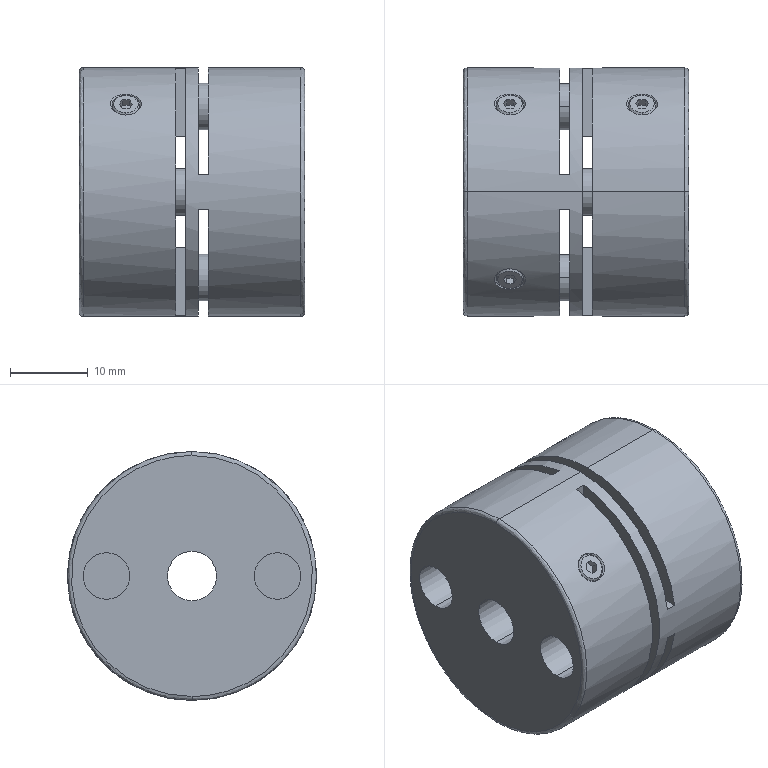Part | STEP file | DBA01-D32-d6.35-e8 | 1 solid | 136 faces | box 29 x 32 x 32 mm | volume 19412 mm3 | plane 64 | cone 36 | cylinder 32 | spline 4 | commonest cylinder face diameters 6 x16 3.242 x8 6.35 x2 8 x2 15 x2 32 x2